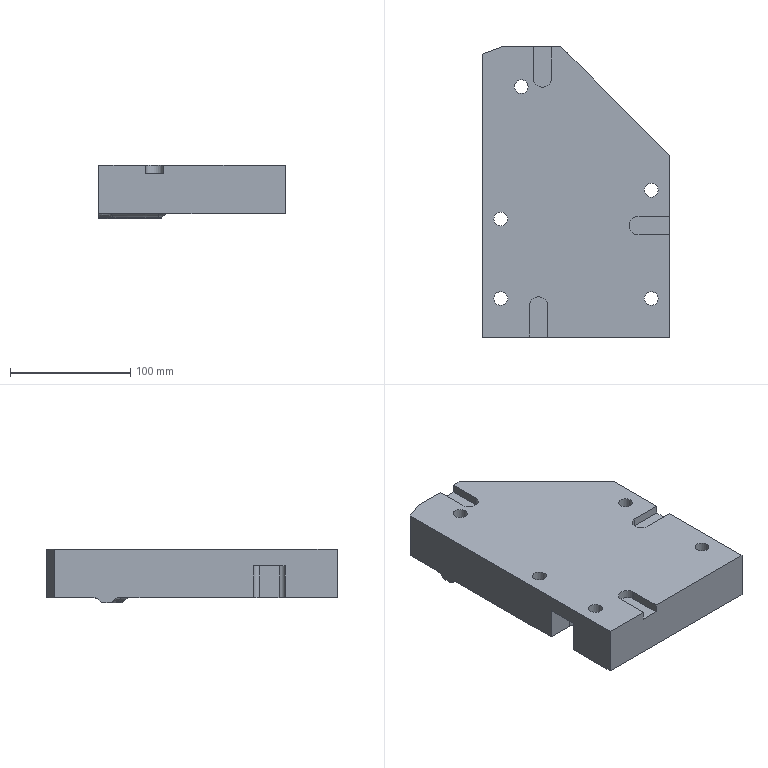Part | NX | features 8 2 | 1 solid | 72 faces | box 155 x 241 x 44.079 mm | volume 1231088 mm3 | plane 36 | cylinder 24 | torus 6 | spline 4 | cone 2 | commonest cylinder face diameters 10 x9 11.5 x5 18 x5 15 x3 8.5 x2